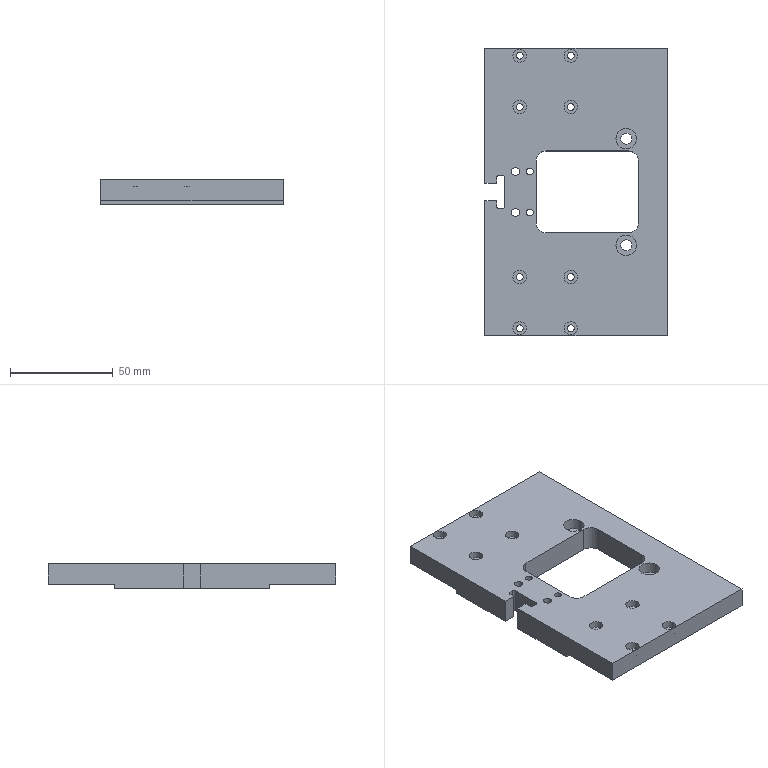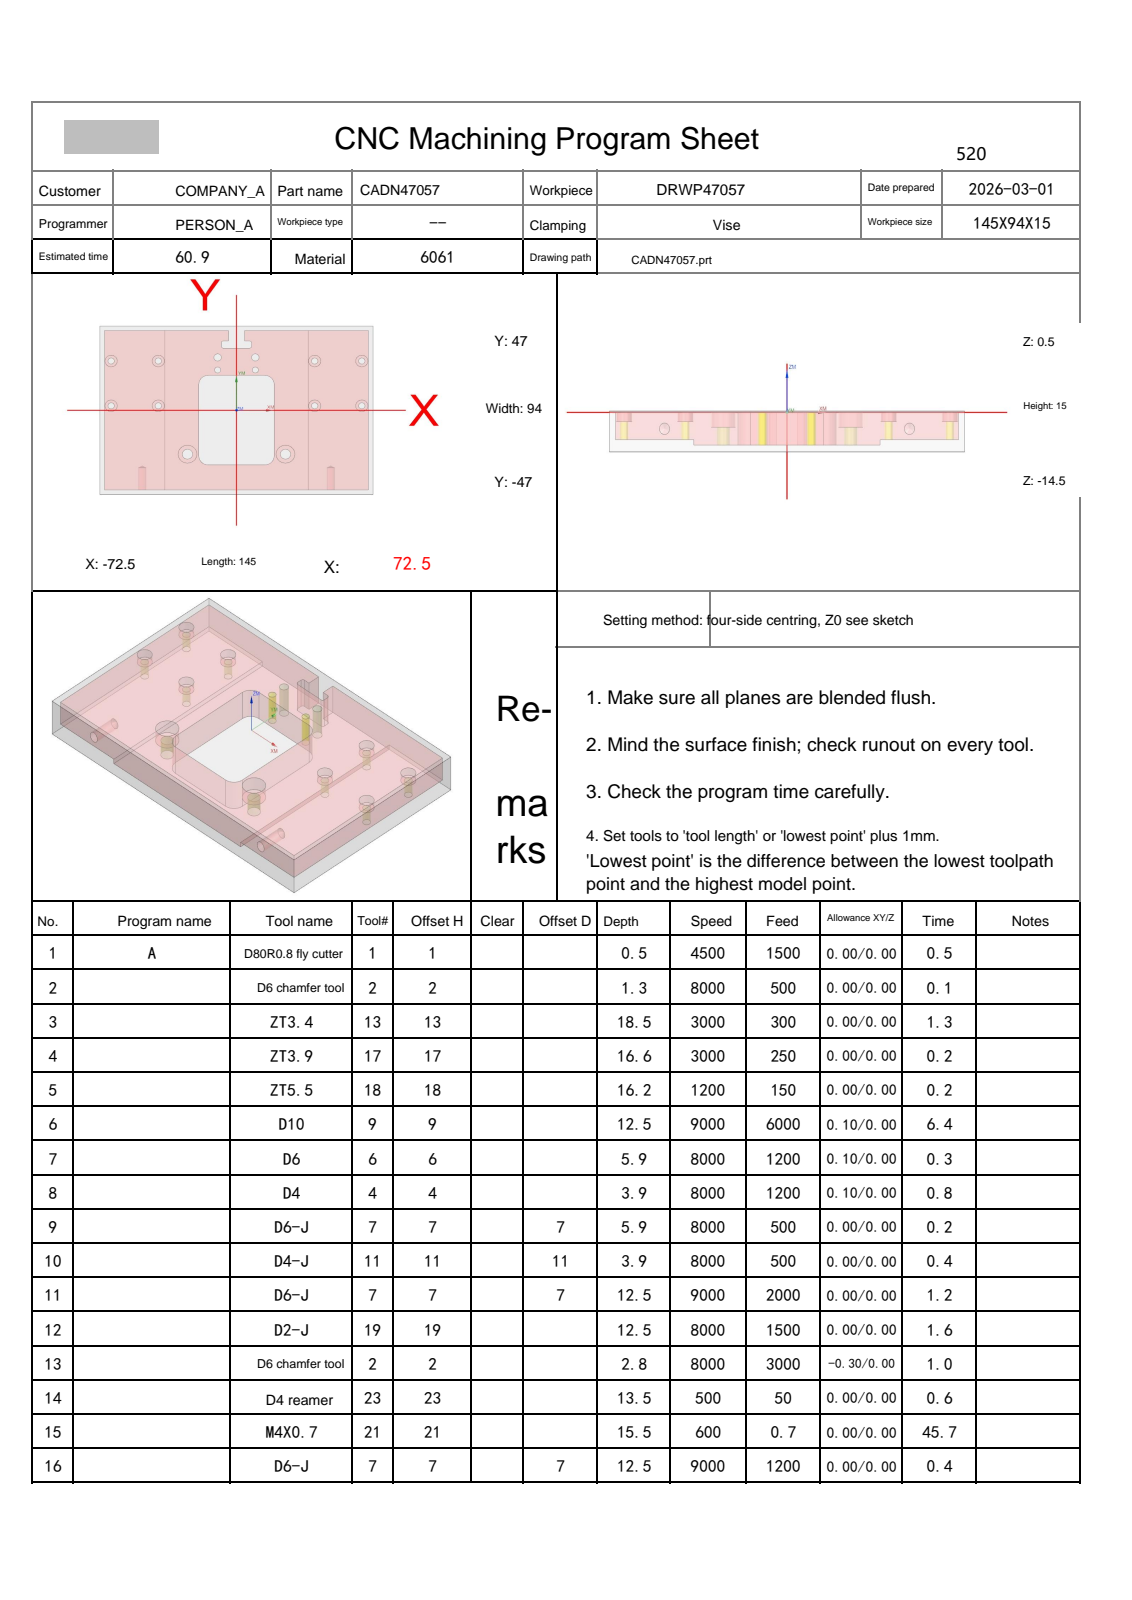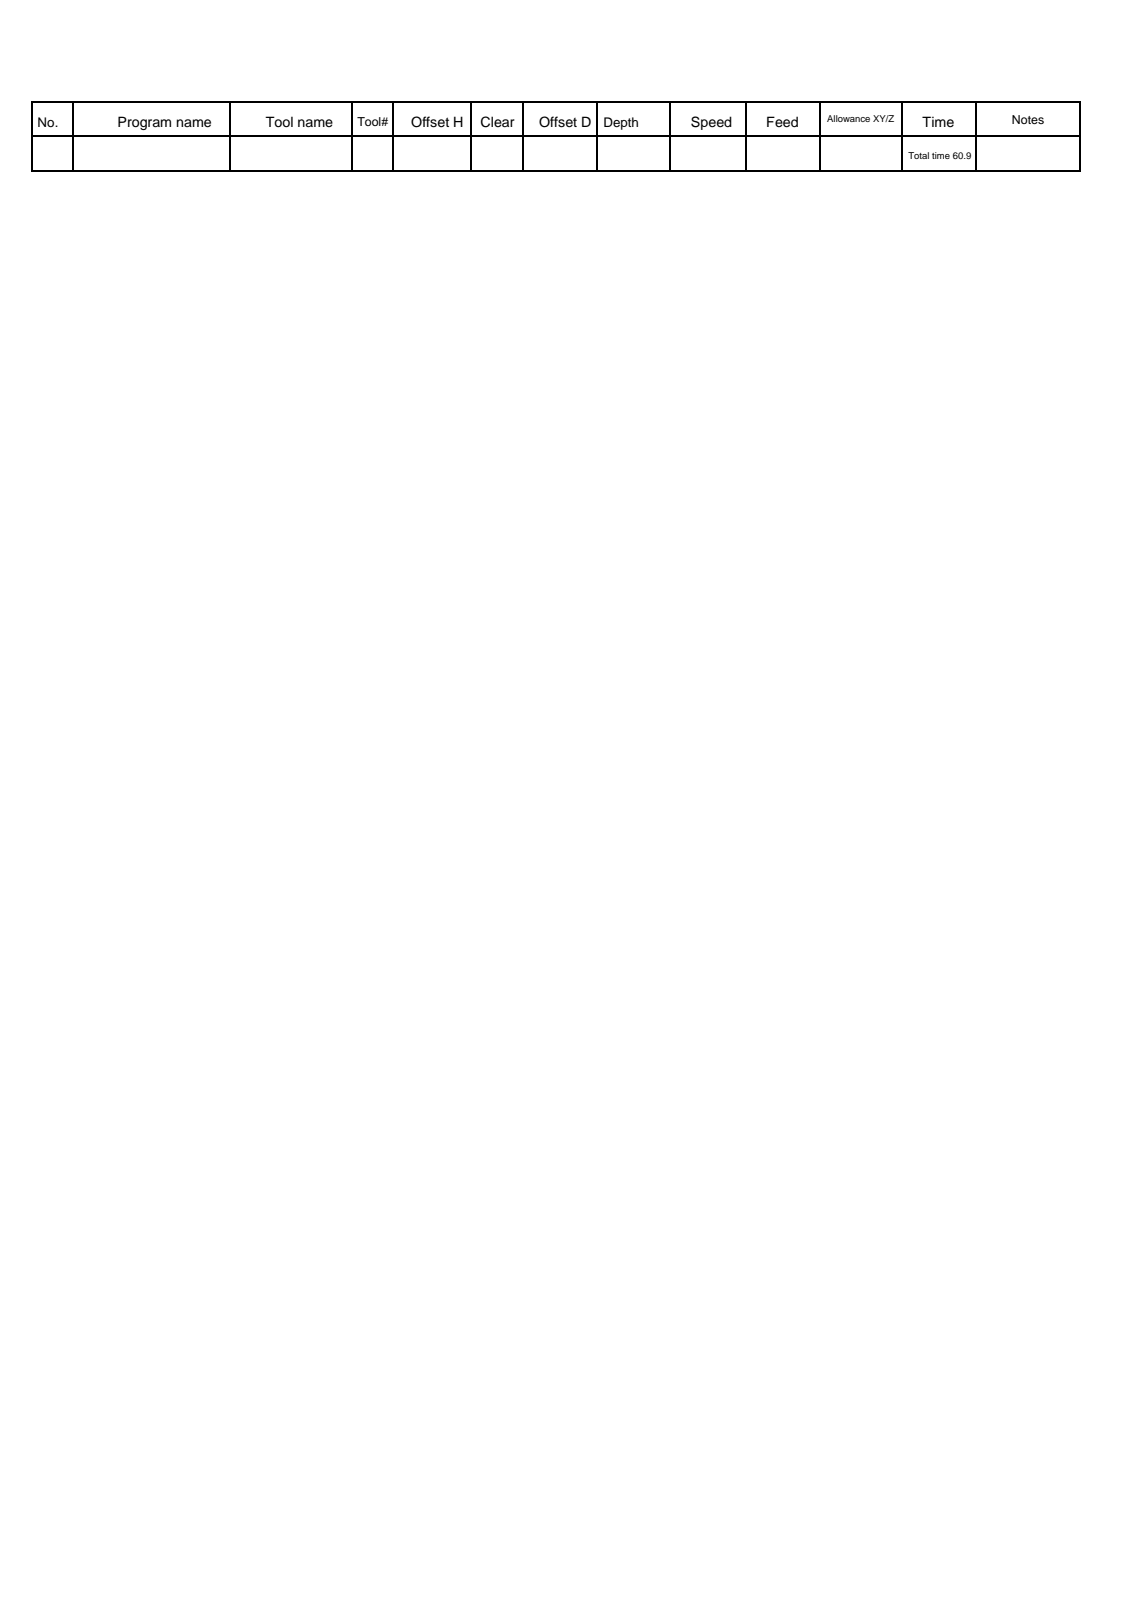NC program | NX | posted by the shop | part box 89 x 140 x 12 mm
Lines 6165 to 6684 of 6684:
N13 T02 M06
(D6 chamfer tool  D=6. R=0. H=02 ce=0.00 di=0.00)
G00 G90 G54 X.25 Y-46.628 M03 S8000
G43 H02 Z50.
M08
Z2.099
G01 Z-1.5 F3000.
G03 X.33 Y-46.328 I-.52 J.3
X.03 Y-45.808 I-.6 J0.0
G01 X0.0 Y-45.8
X-70.
G02 X-71.3 Y-44.5 I0.0 J1.3
G01 Y44.5
G02 X-70. Y45.8 I1.3 J0.0
G01 X-4.25
G02 X-2.95 Y44.5 I0.0 J-1.3
G01 Y38.7
G02 X-4.25 Y37.4 I-1.3 J0.0
G01 X-6.7
Y36.
X6.7
Y37.4
X4.25
G02 X2.95 Y38.7 I0.0 J1.3
G01 Y44.5
G02 X4.25 Y45.8 I1.3 J0.0
G01 X70.
G02 X71.3 Y44.5 I0.0 J-1.3
G01 Y-44.5
G02 X70. Y-45.8 I-1.3 J0.0
G01 X0.0
X-.03 Y-45.808
G03 X-.33 Y-46.328 I.3 J-.52
X-.25 Y-46.628 I.6 J0.0
G01 Z2.099
G00 Z50.
X17.872 Y-5.75
Z2.099
G01 Z-1.5
G03 X18.172 Y-5.83 I.3 J.52
X18.692 Y-5.53 I0.0 J.6
G01 X18.7 Y-5.5
Y14.5
G03 X15. Y18.2 I-3.7 J0.0
G01 X-15.
G03 X-18.7 Y14.5 I0.0 J-3.7
G01 Y-25.5
G03 X-15. Y-29.2 I3.7 J0.0
G01 X15.
G03 X18.7 Y-25.5 I0.0 J3.7
G01 Y-5.5
X18.692 Y-5.47
G03 X18.172 Y-5.17 I-.52 J-.3
X17.872 Y-5.25 I0.0 J-.6
G01 Z2.099
G00 Z50.
G00 G90 X-10. Y22.5 M03 S8000
Z50.
G98 G81 X-10. Y22.5 Z-2.2 R3. F500.
X10.
G80
G00 Z50.
G00 G90 X-10. Y29.5 M03 S8000
Z50.
G98 G81 X-10. Y29.5 Z-2.3 R3. F500.
X10.
G80
G00 Z50.
G00 G90 X67.997 Y29.563 M03 S8000
Z50.
Z2.5
G01 X67.94 Y29.608 Z2.474 F500.
X67.647 Y29.781 Z2.35
X67.334 Y29.913 Z2.226
X67.007 Y30.002 Z2.103
X66.67 Y30.047 Z1.979
X66.33 Z1.855
X65.993 Y30.002 Z1.732
X65.666 Y29.913 Z1.608
X65.353 Y29.781 Z1.484
X65.06 Y29.608 Z1.361
X64.793 Y29.398 Z1.237
X64.556 Y29.155 Z1.113
X64.354 Y28.882 Z.99
X64.23 Y28.668 Z.9
X64.095 Y28.356 Z.776
X64.002 Y28.029 Z.652
X63.954 Y27.693 Z.529
X63.951 Y27.353 Z.405
X63.993 Y27.016 Z.281
X64.08 Y26.688 Z.158
X64.209 Y26.373 Z.034
X64.379 Y26.079 Z-.089
X64.586 Y25.81 Z-.213
X64.828 Y25.571 Z-.337
X65.098 Y25.366 Z-.46
X65.394 Y25.199 Z-.584
X65.71 Y25.072 Z-.708
X66.039 Y24.989 Z-.831
X66.376 Y24.95 Z-.955
X66.5 Z-1.
G03 X69.05 Y27.5 I0.0 J2.55
X66.5 Y30.05 I-2.55 J0.0
X63.95 Y27.5 I0.0 J-2.55
X66.5 Y24.95 I2.55 J0.0
X66.997 Y24.999 I0.0 J2.55
G01 Z1.5
G00 Z50.
X67.997 Y4.563
Z2.5
G01 X67.94 Y4.608 Z2.474
X67.647 Y4.781 Z2.35
X67.334 Y4.913 Z2.226
X67.007 Y5.002 Z2.103
X66.67 Y5.047 Z1.979
X66.33 Z1.855
X65.993 Y5.002 Z1.732
X65.666 Y4.913 Z1.608
X65.353 Y4.781 Z1.484
X65.06 Y4.608 Z1.361
X64.793 Y4.398 Z1.237
X64.556 Y4.155 Z1.113
X64.354 Y3.882 Z.99
X64.23 Y3.668 Z.9
X64.095 Y3.356 Z.776
X64.002 Y3.029 Z.652
X63.954 Y2.693 Z.529
X63.951 Y2.353 Z.405
X63.993 Y2.016 Z.281
X64.08 Y1.688 Z.158
X64.209 Y1.373 Z.034
X64.379 Y1.079 Z-.089
X64.586 Y.81 Z-.213
X64.828 Y.571 Z-.337
X65.098 Y.366 Z-.46
X65.394 Y.199 Z-.584
X65.71 Y.072 Z-.708
X66.039 Y-.011 Z-.831
X66.376 Y-.05 Z-.955
X66.5 Z-1.
G03 X69.05 Y2.5 I0.0 J2.55
X66.5 Y5.05 I-2.55 J0.0
X63.95 Y2.5 I0.0 J-2.55
X66.5 Y-.05 I2.55 J0.0
X66.997 Y-.001 I0.0 J2.55
G01 Z1.5
G00 Z50.
X42.997 Y4.563
Z2.5
G01 X42.94 Y4.608 Z2.474
X42.647 Y4.781 Z2.35
X42.334 Y4.913 Z2.226
X42.007 Y5.002 Z2.103
X41.67 Y5.047 Z1.979
X41.33 Z1.855
X40.993 Y5.002 Z1.732
X40.666 Y4.913 Z1.608
X40.353 Y4.781 Z1.484
X40.06 Y4.608 Z1.361
X39.793 Y4.398 Z1.237
X39.556 Y4.155 Z1.113
X39.354 Y3.882 Z.99
X39.23 Y3.668 Z.9
X39.095 Y3.356 Z.776
X39.002 Y3.029 Z.652
X38.954 Y2.693 Z.529
X38.951 Y2.353 Z.405
X38.993 Y2.016 Z.281
X39.08 Y1.688 Z.158
X39.209 Y1.373 Z.034
X39.379 Y1.079 Z-.089
X39.586 Y.81 Z-.213
X39.828 Y.571 Z-.337
X40.098 Y.366 Z-.46
X40.394 Y.199 Z-.584
X40.71 Y.072 Z-.708
X41.039 Y-.011 Z-.831
X41.376 Y-.05 Z-.955
X41.5 Z-1.
G03 X44.05 Y2.5 I0.0 J2.55
X41.5 Y5.05 I-2.55 J0.0
X38.95 Y2.5 I0.0 J-2.55
X41.5 Y-.05 I2.55 J0.0
X41.997 Y-.001 I0.0 J2.55
G01 Z1.5
G00 Z50.
X42.997 Y29.563
Z2.5
G01 X42.94 Y29.608 Z2.474
X42.647 Y29.781 Z2.35
X42.334 Y29.913 Z2.226
X42.007 Y30.002 Z2.103
X41.67 Y30.047 Z1.979
X41.33 Z1.855
X40.993 Y30.002 Z1.732
X40.666 Y29.913 Z1.608
X40.353 Y29.781 Z1.484
X40.06 Y29.608 Z1.361
X39.793 Y29.398 Z1.237
X39.556 Y29.155 Z1.113
X39.354 Y28.882 Z.99
X39.23 Y28.668 Z.9
X39.095 Y28.356 Z.776
X39.002 Y28.029 Z.652
X38.954 Y27.693 Z.529
X38.951 Y27.353 Z.405
X38.993 Y27.016 Z.281
X39.08 Y26.688 Z.158
X39.209 Y26.373 Z.034
X39.379 Y26.079 Z-.089
X39.586 Y25.81 Z-.213
X39.828 Y25.571 Z-.337
X40.098 Y25.366 Z-.46
X40.394 Y25.199 Z-.584
X40.71 Y25.072 Z-.708
X41.039 Y24.989 Z-.831
X41.376 Y24.95 Z-.955
X41.5 Z-1.
G03 X44.05 Y27.5 I0.0 J2.55
X41.5 Y30.05 I-2.55 J0.0
X38.95 Y27.5 I0.0 J-2.55
X41.5 Y24.95 I2.55 J0.0
X41.997 Y24.999 I0.0 J2.55
G01 Z1.5
G00 Z50.
X-40.003 Y29.563
Z2.5
G01 X-40.06 Y29.608 Z2.474
X-40.353 Y29.781 Z2.35
X-40.666 Y29.913 Z2.226
X-40.993 Y30.002 Z2.103
X-41.33 Y30.047 Z1.979
X-41.67 Z1.855
X-42.007 Y30.002 Z1.732
X-42.334 Y29.913 Z1.608
X-42.647 Y29.781 Z1.484
X-42.94 Y29.608 Z1.361
X-43.207 Y29.398 Z1.237
X-43.444 Y29.155 Z1.113
X-43.647 Y28.882 Z.99
X-43.77 Y28.668 Z.9
X-43.905 Y28.356 Z.776
X-43.998 Y28.029 Z.652
X-44.046 Y27.693 Z.529
X-44.049 Y27.353 Z.405
X-44.007 Y27.016 Z.281
X-43.92 Y26.688 Z.158
X-43.791 Y26.373 Z.034
X-43.621 Y26.079 Z-.089
X-43.414 Y25.81 Z-.213
X-43.172 Y25.571 Z-.337
X-42.902 Y25.366 Z-.46
X-42.606 Y25.199 Z-.584
X-42.29 Y25.072 Z-.708
X-41.961 Y24.989 Z-.831
X-41.624 Y24.95 Z-.955
X-41.5 Z-1.
G03 X-38.95 Y27.5 I0.0 J2.55
X-41.5 Y30.05 I-2.55 J0.0
X-44.05 Y27.5 I0.0 J-2.55
X-41.5 Y24.95 I2.55 J0.0
X-41.003 Y24.999 I0.0 J2.55
G01 Z1.5
G00 Z50.
X-40.003 Y4.563
Z2.5
G01 X-40.06 Y4.608 Z2.474
X-40.353 Y4.781 Z2.35
X-40.666 Y4.913 Z2.226
X-40.993 Y5.002 Z2.103
X-41.33 Y5.047 Z1.979
X-41.67 Z1.855
X-42.007 Y5.002 Z1.732
X-42.334 Y4.913 Z1.608
X-42.647 Y4.781 Z1.484
X-42.94 Y4.608 Z1.361
X-43.207 Y4.398 Z1.237
X-43.444 Y4.155 Z1.113
X-43.647 Y3.882 Z.99
X-43.77 Y3.668 Z.9
X-43.905 Y3.356 Z.776
X-43.998 Y3.029 Z.652
X-44.046 Y2.693 Z.529
X-44.049 Y2.353 Z.405
X-44.007 Y2.016 Z.281
X-43.92 Y1.688 Z.158
X-43.791 Y1.373 Z.034
X-43.621 Y1.079 Z-.089
X-43.414 Y.81 Z-.213
X-43.172 Y.571 Z-.337
X-42.902 Y.366 Z-.46
X-42.606 Y.199 Z-.584
X-42.29 Y.072 Z-.708
X-41.961 Y-.011 Z-.831
X-41.624 Y-.05 Z-.955
X-41.5 Z-1.
G03 X-38.95 Y2.5 I0.0 J2.55
X-41.5 Y5.05 I-2.55 J0.0
X-44.05 Y2.5 I0.0 J-2.55
X-41.5 Y-.05 I2.55 J0.0
X-41.003 Y-.001 I0.0 J2.55
G01 Z1.5
G00 Z50.
X-65.003 Y4.563
Z2.5
G01 X-65.06 Y4.608 Z2.474
X-65.353 Y4.781 Z2.35
X-65.666 Y4.913 Z2.226
X-65.993 Y5.002 Z2.103
X-66.33 Y5.047 Z1.979
X-66.67 Z1.855
X-67.007 Y5.002 Z1.732
X-67.334 Y4.913 Z1.608
X-67.647 Y4.781 Z1.484
X-67.94 Y4.608 Z1.361
X-68.207 Y4.398 Z1.237
X-68.444 Y4.155 Z1.113
X-68.647 Y3.882 Z.99
X-68.77 Y3.668 Z.9
X-68.905 Y3.356 Z.776
X-68.998 Y3.029 Z.652
X-69.046 Y2.693 Z.529
X-69.049 Y2.353 Z.405
X-69.007 Y2.016 Z.281
X-68.92 Y1.688 Z.158
X-68.791 Y1.373 Z.034
X-68.621 Y1.079 Z-.089
X-68.414 Y.81 Z-.213
X-68.172 Y.571 Z-.337
X-67.902 Y.366 Z-.46
X-67.606 Y.199 Z-.584
X-67.29 Y.072 Z-.708
X-66.961 Y-.011 Z-.831
X-66.624 Y-.05 Z-.955
X-66.5 Z-1.
G03 X-63.95 Y2.5 I0.0 J2.55
X-66.5 Y5.05 I-2.55 J0.0
X-69.05 Y2.5 I0.0 J-2.55
X-66.5 Y-.05 I2.55 J0.0
X-66.003 Y-.001 I0.0 J2.55
G01 Z1.5
G00 Z50.
X-65.003 Y29.563
Z2.5
G01 X-65.06 Y29.608 Z2.474
X-65.353 Y29.781 Z2.35
X-65.666 Y29.913 Z2.226
X-65.993 Y30.002 Z2.103
X-66.33 Y30.047 Z1.979
X-66.67 Z1.855
X-67.007 Y30.002 Z1.732
X-67.334 Y29.913 Z1.608
X-67.647 Y29.781 Z1.484
X-67.94 Y29.608 Z1.361
X-68.207 Y29.398 Z1.237
X-68.444 Y29.155 Z1.113
X-68.647 Y28.882 Z.99
X-68.77 Y28.668 Z.9
X-68.905 Y28.356 Z.776
X-68.998 Y28.029 Z.652
X-69.046 Y27.693 Z.529
X-69.049 Y27.353 Z.405
X-69.007 Y27.016 Z.281
X-68.92 Y26.688 Z.158
X-68.791 Y26.373 Z.034
X-68.621 Y26.079 Z-.089
X-68.414 Y25.81 Z-.213
X-68.172 Y25.571 Z-.337
X-67.902 Y25.366 Z-.46
X-67.606 Y25.199 Z-.584
X-67.29 Y25.072 Z-.708
X-66.961 Y24.989 Z-.831
X-66.624 Y24.95 Z-.955
X-66.5 Z-1.
G03 X-63.95 Y27.5 I0.0 J2.55
X-66.5 Y30.05 I-2.55 J0.0
X-69.05 Y27.5 I0.0 J-2.55
X-66.5 Y24.95 I2.55 J0.0
X-66.003 Y24.999 I0.0 J2.55
G01 Z1.5
G00 Z50.
G00 G90 X-29.386 Y-21.846 M03 S8000
Z50.
Z2.5
G01 X-29.394 Y-21.855 Z2.495 F800.
X-29.644 Y-22.211 Z2.337
X-29.804 Y-22.489 Z2.22
X-29.988 Y-22.883 Z2.062
X-30.13 Y-23.293 Z1.904
X-30.231 Y-23.716 Z1.746
X-30.288 Y-24.146 Z1.588
X-30.302 Y-24.58 Z1.43
X-30.272 Y-25.014 Z1.272
X-30.199 Y-25.442 Z1.114
X-30.082 Y-25.86 Z.956
X-29.924 Y-26.265 Z.797
X-29.727 Y-26.652 Z.639
X-29.491 Y-27.016 Z.481
X-29.219 Y-27.355 Z.323
X-28.915 Y-27.665 Z.165
X-28.581 Y-27.943 Z.007
X-28.221 Y-28.186 Z-.151
X-27.838 Y-28.391 Z-.309
X-27.436 Y-28.556 Z-.467
X-27.02 Y-28.68 Z-.625
X-26.593 Y-28.762 Z-.783
X-26.161 Y-28.8 Z-.942
X-26. Z-1.
G03 X-21.7 Y-24.5 I0.0 J4.3
X-26. Y-20.2 I-4.3 J0.0
X-30.3 Y-24.5 I0.0 J-4.3
X-26. Y-28.8 I4.3 J0.0
X-25.501 Y-28.771 I0.0 J4.3
G01 Z1.5
G00 Z50.
X22.614 Y-21.846
Z2.5
G01 X22.606 Y-21.855 Z2.495
X22.356 Y-22.211 Z2.337
X22.196 Y-22.489 Z2.22
X22.012 Y-22.883 Z2.062
X21.87 Y-23.293 Z1.904
X21.769 Y-23.716 Z1.746
X21.712 Y-24.146 Z1.588
X21.698 Y-24.58 Z1.43
X21.728 Y-25.014 Z1.272
X21.801 Y-25.442 Z1.114
X21.918 Y-25.86 Z.956
X22.076 Y-26.265 Z.797
X22.273 Y-26.652 Z.639
X22.509 Y-27.016 Z.481
X22.781 Y-27.355 Z.323
X23.085 Y-27.665 Z.165
X23.419 Y-27.943 Z.007
X23.779 Y-28.186 Z-.151
X24.162 Y-28.391 Z-.309
X24.564 Y-28.556 Z-.467
X24.98 Y-28.68 Z-.625
X25.407 Y-28.762 Z-.783
X25.839 Y-28.8 Z-.942
X26. Z-1.
G03 X30.3 Y-24.5 I0.0 J4.3
X26. Y-20.2 I-4.3 J0.0
X21.7 Y-24.5 I0.0 J-4.3
X26. Y-28.8 I4.3 J0.0
X26.499 Y-28.771 I0.0 J4.3
G01 Z1.5
G00 Z50.
G91 G28 Z0.0
M05
M09
G91 G28 Z0.0
M01
N14 T23 M06
(D4 reamer D=4. DR_a=180 H=23)
G00 G90 G54 X-10. Y29.5 M03 S500
G43 H23 Z50.
M08
G98 G81 X-10. Y29.5 Z-13. R1. F50.
X10.
G80
G00 Z50.
G91 G28 Z0.0
M05
M09
G91 G28 Z0.0
M01
N15 T21 M06
(M4X0.7 D=3.3 DR_a=180 H=21)
G00 G90 G54 X-10. Y22.5 M03 S600
G43 H21 Z50.
M08
G95
G98 G84 X-10. Y22.5 Z-15. R1. F.7 Q4.
X10.
G80
G94
G00 Z50.
G91 G28 Z0.0
M05
M09
G91 G28 Z0.0
M01
N16 T07 M06
(D6-J  D=6. R=0. H=07 ce=0.00 di=0.00)
G00 G90 G54 X71.017 Y-48.573 M03 S9000
G43 H07 Z50.
M08
Z-11.5
G01 Z-12. F1200.
G41 D07
X70.992 Y-48.375
G03 X70. Y-47.5 I-.992 J-.125
G01 X-70.
G02 X-73. Y-44.5 I0.0 J3.
G01 Y44.5
G02 X-70. Y47.5 I3. J0.0
G01 X-4.25
G02 X-1.25 Y44.5 I0.0 J-3.
G01 Y38.7
G02 X-1.422 Y37.7 I-3. J0.0
G01 X1.422
G02 X1.25 Y38.7 I2.828 J1.
G01 Y44.5
G02 X4.25 Y47.5 I3. J0.0
G01 X70.
G02 X73. Y44.5 I0.0 J-3.
G01 Y-44.5
G02 X70. Y-47.5 I-3. J0.0
G01 X69.5
G03 X68.5 Y-48.5 I0.0 J-1.
G01 G40 Y-48.7
Z-11.5
G00 Z50.
M05
M09
G91 G28 Z0.0
G91 G28 Y0.0
M30
%